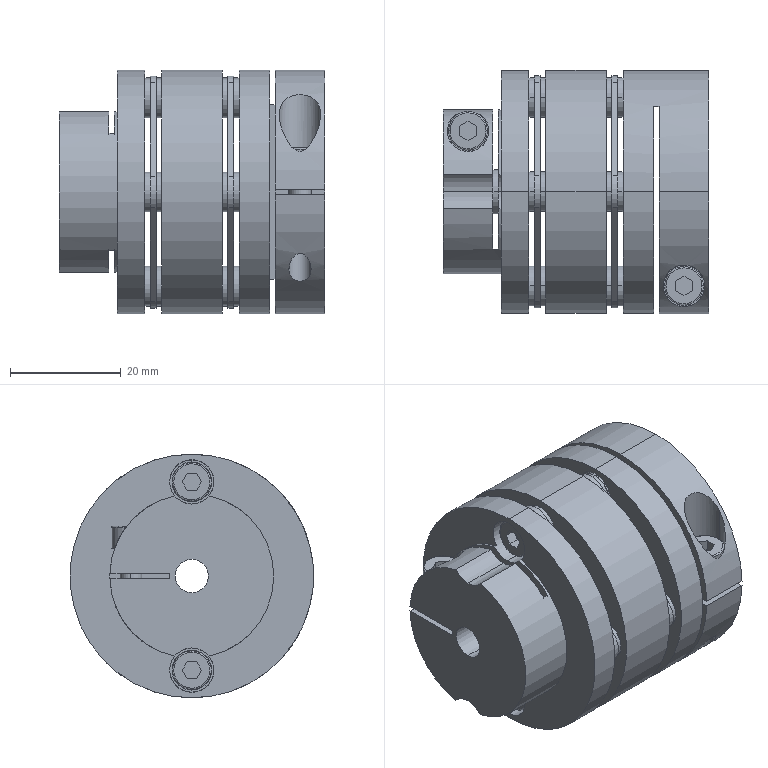Part | STEP file | SFC-040DA2-6B-16B_2_03 | 1 solid | 211 faces | box 48 x 44 x 44 mm | volume 46226 mm3 | cylinder 109 | plane 86 | spline 12 | cone 4 | commonest cylinder face diameters 7.2 x32 8 x27 7 x12 4 x8 44 x8 7.5 x5